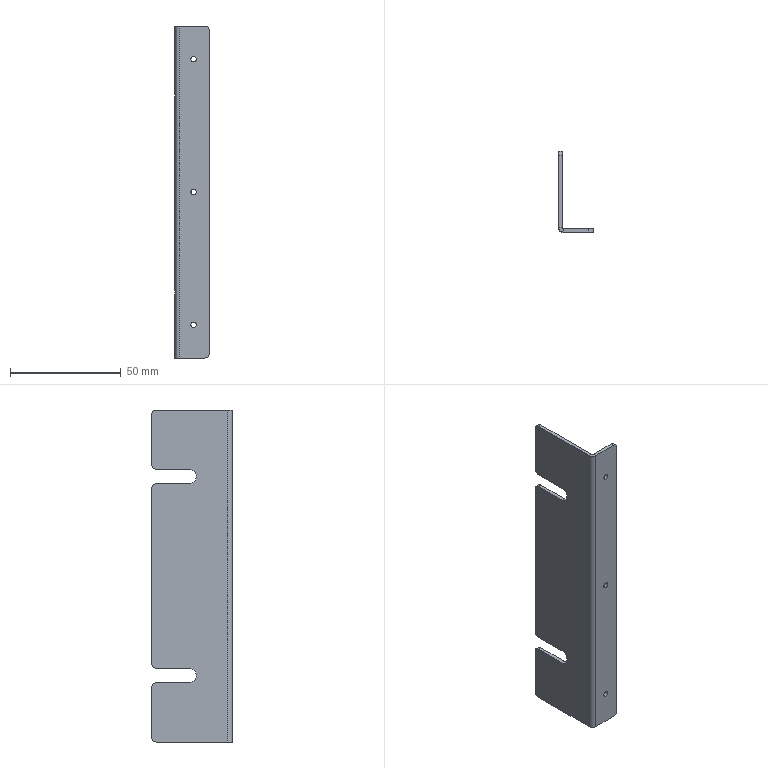Part | STEP file | Sheet-metal door stop plate | 1 solid | 36 faces | box 15.5 x 36.5 x 150 mm | volume 10828 mm3 | cylinder 18 | plane 18 | commonest cylinder face diameters 4 x9 2.5 x6 6.5 x2 1 x1